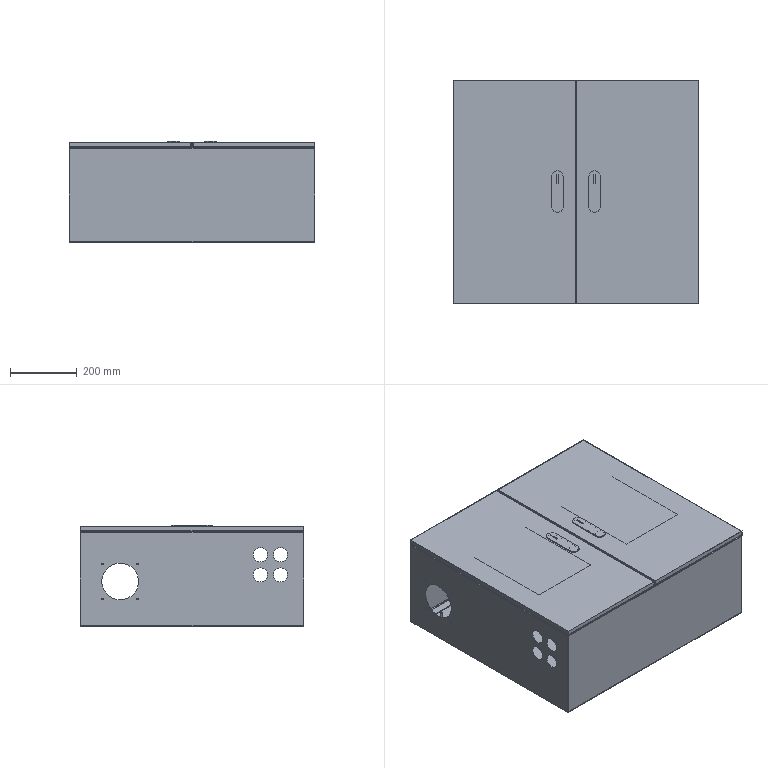Part | SolidWorks | features AEMSimFeature 1, MirrorCompFeat 1, ReferencePattern 1 | 8 solids | 330 faces | box 736 x 670 x 303 mm | volume 3762894 mm3 | plane 172 | cylinder 126 | spline 32 | commonest cylinder face diameters 42 x28 7 x20 5 x16 4 x12 6 x12 1.473 x6